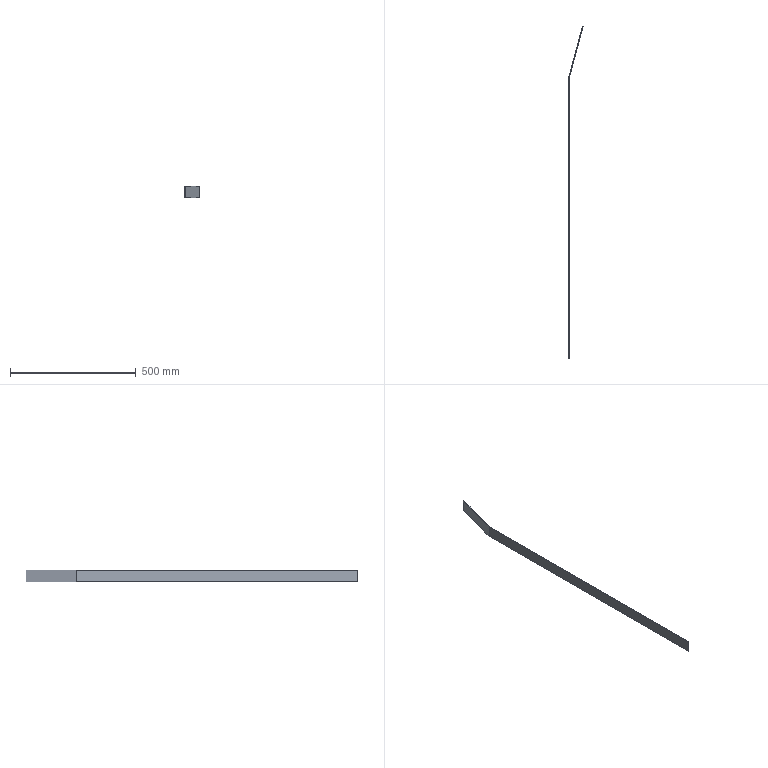Part | STEP file | SN10_016_001-01_CHAPA | 1 solid | 10 faces | box 56.488 x 1320 x 45 mm | volume 179098 mm3 | plane 8 | cylinder 2 | commonest cylinder face diameters 6 x1 12 x1
STEP:
#1=CARTESIAN_POINT('',(0.,0.,0.));
#2=DIRECTION('',(0.,0.,1.));
#3=DIRECTION('',(1.,0.,0.));
#4=AXIS2_PLACEMENT_3D('',#1,#2,#3);
#5=CARTESIAN_POINT('',(5319.204,-379.237,95.));
#6=VERTEX_POINT('',#5);
#7=CARTESIAN_POINT('',(5372.59,-180.,95.));
#8=VERTEX_POINT('',#7);
#9=CARTESIAN_POINT('',(5319.204,-379.237,95.));
#10=DIRECTION('',(0.2588,0.9659,0.));
#11=VECTOR('',#10,1.);
#12=LINE('',#9,#11);
#13=CARTESIAN_POINT('',(5319.204,-379.237,45.));
#14=DIRECTION('',(0.9659,-0.2588,0.));
#15=DIRECTION('',(0.,0.,-1.));
#16=AXIS2_PLACEMENT_3D('',#13,#14,#15);
#17=PLANE('',#16);
#18=CARTESIAN_POINT('',(-50.,0.));
#19=DIRECTION('',(0.,1.));
#20=VECTOR('',#19,1.);
#21=LINE('',#18,#20);
#22=(GEOMETRIC_REPRESENTATION_CONTEXT(2)PARAMETRIC_REPRESENTATION_CONTEXT()REPRESENTATION_CONTEXT('',''));
#23=DEFINITIONAL_REPRESENTATION('',(#21),#22);
#24=PCURVE('',#17,#23);
#25=CARTESIAN_POINT('',(0.,0.,95.));
#26=DIRECTION('',(0.,0.,1.));
#27=DIRECTION('',(1.,0.,0.));
#28=AXIS2_PLACEMENT_3D('',#25,#26,#27);
#29=PLANE('',#28);
#30=CARTESIAN_POINT('',(5319.204,-379.237));
#31=DIRECTION('',(0.2588,0.9659));
#32=VECTOR('',#31,1.);
#33=LINE('',#30,#32);
#34=(GEOMETRIC_REPRESENTATION_CONTEXT(2)PARAMETRIC_REPRESENTATION_CONTEXT()REPRESENTATION_CONTEXT('',''));
#35=DEFINITIONAL_REPRESENTATION('',(#33),#34);
#36=PCURVE('',#29,#35);
#37=SURFACE_CURVE('',#12,(#24,#36),.PCURVE_S1.);
#38=EDGE_CURVE('',#6,#8,#37,.T.);
#39=ORIENTED_EDGE('',*,*,#38,.T.);
#40=CARTESIAN_POINT('',(5372.59,-180.,50.));
#41=VERTEX_POINT('',#40);
#42=CARTESIAN_POINT('',(5372.59,-180.,50.));
#43=DIRECTION('',(0.,0.,1.));
#44=VECTOR('',#43,1.);
#45=LINE('',#42,#44);
#46=CARTESIAN_POINT('',(-5.,206.265));
#47=DIRECTION('',(-1.,0.));
#48=VECTOR('',#47,1.);
#49=LINE('',#46,#48);
#50=(GEOMETRIC_REPRESENTATION_CONTEXT(2)PARAMETRIC_REPRESENTATION_CONTEXT()REPRESENTATION_CONTEXT('',''));
#51=DEFINITIONAL_REPRESENTATION('',(#49),#50);
#52=PCURVE('',#17,#51);
#53=CARTESIAN_POINT('',(5375.488,-180.776,45.));
#54=DIRECTION('',(0.2588,0.9659,0.));
#55=DIRECTION('',(0.,0.,1.));
#56=AXIS2_PLACEMENT_3D('',#53,#54,#55);
#57=PLANE('',#56);
#58=CARTESIAN_POINT('',(5.,-3.));
#59=DIRECTION('',(1.,0.));
#60=VECTOR('',#59,1.);
#61=LINE('',#58,#60);
#62=(GEOMETRIC_REPRESENTATION_CONTEXT(2)PARAMETRIC_REPRESENTATION_CONTEXT()REPRESENTATION_CONTEXT('',''));
#63=DEFINITIONAL_REPRESENTATION('',(#61),#62);
#64=PCURVE('',#57,#63);
#65=SURFACE_CURVE('',#45,(#52,#64),.PCURVE_S1.);
#66=EDGE_CURVE('',#41,#8,#65,.T.);
#67=ORIENTED_EDGE('',*,*,#66,.F.);
#68=CARTESIAN_POINT('',(5319.204,-379.237,50.));
#69=VERTEX_POINT('',#68);
#70=CARTESIAN_POINT('',(5319.204,-379.237,50.));
#71=DIRECTION('',(0.2588,0.9659,0.));
#72=VECTOR('',#71,1.);
#73=LINE('',#70,#72);
#74=CARTESIAN_POINT('',(-5.,0.));
#75=DIRECTION('',(0.,1.));
#76=VECTOR('',#75,1.);
#77=LINE('',#74,#76);
#78=(GEOMETRIC_REPRESENTATION_CONTEXT(2)PARAMETRIC_REPRESENTATION_CONTEXT()REPRESENTATION_CONTEXT('',''));
#79=DEFINITIONAL_REPRESENTATION('',(#77),#78);
#80=PCURVE('',#17,#79);
#81=CARTESIAN_POINT('',(0.,0.,50.));
#82=DIRECTION('',(0.,0.,1.));
#83=DIRECTION('',(1.,0.,0.));
#84=AXIS2_PLACEMENT_3D('',#81,#82,#83);
#85=PLANE('',#84);
#86=CARTESIAN_POINT('',(5319.204,-379.237));
#87=DIRECTION('',(0.2588,0.9659));
#88=VECTOR('',#87,1.);
#89=LINE('',#86,#88);
#90=(GEOMETRIC_REPRESENTATION_CONTEXT(2)PARAMETRIC_REPRESENTATION_CONTEXT()REPRESENTATION_CONTEXT('',''));
#91=DEFINITIONAL_REPRESENTATION('',(#89),#90);
#92=PCURVE('',#85,#91);
#93=SURFACE_CURVE('',#73,(#80,#92),.PCURVE_S1.);
#94=EDGE_CURVE('',#69,#41,#93,.T.);
#95=ORIENTED_EDGE('',*,*,#94,.F.);
#96=CARTESIAN_POINT('',(5319.204,-379.237,50.));
#97=DIRECTION('',(0.,0.,1.));
#98=VECTOR('',#97,1.);
#99=LINE('',#96,#98);
#100=CARTESIAN_POINT('',(-5.,0.));
#101=DIRECTION('',(-1.,0.));
#102=VECTOR('',#101,1.);
#103=LINE('',#100,#102);
#104=(GEOMETRIC_REPRESENTATION_CONTEXT(2)PARAMETRIC_REPRESENTATION_CONTEXT()REPRESENTATION_CONTEXT('',''));
#105=DEFINITIONAL_REPRESENTATION('',(#103),#104);
#106=PCURVE('',#17,#105);
#107=CARTESIAN_POINT('',(5325.,-380.79,72.5));
#108=DIRECTION('',(0.,0.,1.));
#109=DIRECTION('',(-0.9659,0.2588,0.));
#110=AXIS2_PLACEMENT_3D('',#107,#108,#109);
#111=CYLINDRICAL_SURFACE('',#110,6.);
#112=CARTESIAN_POINT('',(0.,-22.5));
#113=DIRECTION('',(0.,1.));
#114=VECTOR('',#113,1.);
#115=LINE('',#112,#114);
#116=(GEOMETRIC_REPRESENTATION_CONTEXT(2)PARAMETRIC_REPRESENTATION_CONTEXT()REPRESENTATION_CONTEXT('',''));
#117=DEFINITIONAL_REPRESENTATION('',(#115),#116);
#118=PCURVE('',#111,#117);
#119=SURFACE_CURVE('',#99,(#106,#118),.PCURVE_S1.);
#120=EDGE_CURVE('',#69,#6,#119,.T.);
#121=ORIENTED_EDGE('',*,*,#120,.T.);
#122=EDGE_LOOP('',(#39,#67,#95,#121));
#123=FACE_BOUND('',#122,.T.);
#124=ADVANCED_FACE('',(#123),#17,.F.);
#125=ORIENTED_EDGE('',*,*,#120,.F.);
#126=CARTESIAN_POINT('',(5319.,-380.79,50.));
#127=VERTEX_POINT('',#126);
#128=CARTESIAN_POINT('',(5325.,-380.79,50.));
#129=DIRECTION('',(0.,0.,1.));
#130=DIRECTION('',(1.,0.,0.));
#131=AXIS2_PLACEMENT_3D('',#128,#129,#130);
#132=CIRCLE('',#131,6.);
#133=CARTESIAN_POINT('',(-2.88,-22.5));
#134=DIRECTION('',(1.,0.));
#135=VECTOR('',#134,1.);
#136=LINE('',#133,#135);
#137=(GEOMETRIC_REPRESENTATION_CONTEXT(2)PARAMETRIC_REPRESENTATION_CONTEXT()REPRESENTATION_CONTEXT('',''));
#138=DEFINITIONAL_REPRESENTATION('',(#136),#137);
#139=PCURVE('',#111,#138);
#140=CARTESIAN_POINT('',(5325.,-380.79));
#141=DIRECTION('',(1.,0.));
#142=AXIS2_PLACEMENT_2D('',#140,#141);
#143=CIRCLE('',#142,6.);
#144=(GEOMETRIC_REPRESENTATION_CONTEXT(2)PARAMETRIC_REPRESENTATION_CONTEXT()REPRESENTATION_CONTEXT('',''));
#145=DEFINITIONAL_REPRESENTATION('',(#143),#144);
#146=PCURVE('',#85,#145);
#147=SURFACE_CURVE('',#132,(#139,#146),.PCURVE_S1.);
#148=EDGE_CURVE('',#69,#127,#147,.T.);
#149=ORIENTED_EDGE('',*,*,#148,.T.);
#150=CARTESIAN_POINT('',(5319.,-380.79,95.));
#151=VERTEX_POINT('',#150);
#152=CARTESIAN_POINT('',(5319.,-380.79,50.));
#153=DIRECTION('',(0.,0.,1.));
#154=VECTOR('',#153,1.);
#155=LINE('',#152,#154);
#156=CARTESIAN_POINT('',(0.2618,-22.5));
#157=DIRECTION('',(0.,1.));
#158=VECTOR('',#157,1.);
#159=LINE('',#156,#158);
#160=(GEOMETRIC_REPRESENTATION_CONTEXT(2)PARAMETRIC_REPRESENTATION_CONTEXT()REPRESENTATION_CONTEXT('',''));
#161=DEFINITIONAL_REPRESENTATION('',(#159),#160);
#162=PCURVE('',#111,#161);
#163=CARTESIAN_POINT('',(5319.,-1500.,45.));
#164=DIRECTION('',(1.,0.,0.));
#165=DIRECTION('',(0.,0.,-1.));
#166=AXIS2_PLACEMENT_3D('',#163,#164,#165);
#167=PLANE('',#166);
#168=CARTESIAN_POINT('',(-5.,1119.21));
#169=DIRECTION('',(-1.,0.));
#170=VECTOR('',#169,1.);
#171=LINE('',#168,#170);
#172=(GEOMETRIC_REPRESENTATION_CONTEXT(2)PARAMETRIC_REPRESENTATION_CONTEXT()REPRESENTATION_CONTEXT('',''));
#173=DEFINITIONAL_REPRESENTATION('',(#171),#172);
#174=PCURVE('',#167,#173);
#175=SURFACE_CURVE('',#155,(#162,#174),.PCURVE_S1.);
#176=EDGE_CURVE('',#127,#151,#175,.T.);
#177=ORIENTED_EDGE('',*,*,#176,.T.);
#178=CARTESIAN_POINT('',(5325.,-380.79,95.));
#179=DIRECTION('',(0.,0.,1.));
#180=DIRECTION('',(1.,0.,0.));
#181=AXIS2_PLACEMENT_3D('',#178,#179,#180);
#182=CIRCLE('',#181,6.);
#183=CARTESIAN_POINT('',(-2.88,22.5));
#184=DIRECTION('',(1.,0.));
#185=VECTOR('',#184,1.);
#186=LINE('',#183,#185);
#187=(GEOMETRIC_REPRESENTATION_CONTEXT(2)PARAMETRIC_REPRESENTATION_CONTEXT()REPRESENTATION_CONTEXT('',''));
#188=DEFINITIONAL_REPRESENTATION('',(#186),#187);
#189=PCURVE('',#111,#188);
#190=CARTESIAN_POINT('',(5325.,-380.79));
#191=DIRECTION('',(1.,0.));
#192=AXIS2_PLACEMENT_2D('',#190,#191);
#193=CIRCLE('',#192,6.);
#194=(GEOMETRIC_REPRESENTATION_CONTEXT(2)PARAMETRIC_REPRESENTATION_CONTEXT()REPRESENTATION_CONTEXT('',''));
#195=DEFINITIONAL_REPRESENTATION('',(#193),#194);
#196=PCURVE('',#29,#195);
#197=SURFACE_CURVE('',#182,(#189,#196),.PCURVE_S1.);
#198=EDGE_CURVE('',#6,#151,#197,.T.);
#199=ORIENTED_EDGE('',*,*,#198,.F.);
#200=EDGE_LOOP('',(#125,#149,#177,#199));
#201=FACE_BOUND('',#200,.T.);
#202=ADVANCED_FACE('',(#201),#111,.T.);
#203=CARTESIAN_POINT('',(5319.,-1500.,95.));
#204=VERTEX_POINT('',#203);
#205=CARTESIAN_POINT('',(5319.,-1500.,95.));
#206=DIRECTION('',(0.,1.,0.));
#207=VECTOR('',#206,1.);
#208=LINE('',#205,#207);
#209=CARTESIAN_POINT('',(-50.,0.));
#210=DIRECTION('',(0.,1.));
#211=VECTOR('',#210,1.);
#212=LINE('',#209,#211);
#213=(GEOMETRIC_REPRESENTATION_CONTEXT(2)PARAMETRIC_REPRESENTATION_CONTEXT()REPRESENTATION_CONTEXT('',''));
#214=DEFINITIONAL_REPRESENTATION('',(#212),#213);
#215=PCURVE('',#167,#214);
#216=CARTESIAN_POINT('',(5319.,-1500.));
#217=DIRECTION('',(0.,1.));
#218=VECTOR('',#217,1.);
#219=LINE('',#216,#218);
#220=(GEOMETRIC_REPRESENTATION_CONTEXT(2)PARAMETRIC_REPRESENTATION_CONTEXT()REPRESENTATION_CONTEXT('',''));
#221=DEFINITIONAL_REPRESENTATION('',(#219),#220);
#222=PCURVE('',#29,#221);
#223=SURFACE_CURVE('',#208,(#215,#222),.PCURVE_S1.);
#224=EDGE_CURVE('',#204,#151,#223,.T.);
#225=ORIENTED_EDGE('',*,*,#224,.T.);
#226=ORIENTED_EDGE('',*,*,#176,.F.);
#227=CARTESIAN_POINT('',(5319.,-1500.,50.));
#228=VERTEX_POINT('',#227);
#229=CARTESIAN_POINT('',(5319.,-1500.,50.));
#230=DIRECTION('',(0.,1.,0.));
#231=VECTOR('',#230,1.);
#232=LINE('',#229,#231);
#233=CARTESIAN_POINT('',(-5.,0.));
#234=DIRECTION('',(0.,1.));
#235=VECTOR('',#234,1.);
#236=LINE('',#233,#235);
#237=(GEOMETRIC_REPRESENTATION_CONTEXT(2)PARAMETRIC_REPRESENTATION_CONTEXT()REPRESENTATION_CONTEXT('',''));
#238=DEFINITIONAL_REPRESENTATION('',(#236),#237);
#239=PCURVE('',#167,#238);
#240=CARTESIAN_POINT('',(5319.,-1500.));
#241=DIRECTION('',(0.,1.));
#242=VECTOR('',#241,1.);
#243=LINE('',#240,#242);
#244=(GEOMETRIC_REPRESENTATION_CONTEXT(2)PARAMETRIC_REPRESENTATION_CONTEXT()REPRESENTATION_CONTEXT('',''));
#245=DEFINITIONAL_REPRESENTATION('',(#243),#244);
#246=PCURVE('',#85,#245);
#247=SURFACE_CURVE('',#232,(#239,#246),.PCURVE_S1.);
#248=EDGE_CURVE('',#228,#127,#247,.T.);
#249=ORIENTED_EDGE('',*,*,#248,.F.);
#250=CARTESIAN_POINT('',(5319.,-1500.,50.));
#251=DIRECTION('',(0.,0.,1.));
#252=VECTOR('',#251,1.);
#253=LINE('',#250,#252);
#254=CARTESIAN_POINT('',(-5.,0.));
#255=DIRECTION('',(-1.,0.));
#256=VECTOR('',#255,1.);
#257=LINE('',#254,#256);
#258=(GEOMETRIC_REPRESENTATION_CONTEXT(2)PARAMETRIC_REPRESENTATION_CONTEXT()REPRESENTATION_CONTEXT('',''));
#259=DEFINITIONAL_REPRESENTATION('',(#257),#258);
#260=PCURVE('',#167,#259);
#261=CARTESIAN_POINT('',(5319.,-1500.,45.));
#262=DIRECTION('',(0.,-1.,0.));
#263=DIRECTION('',(0.,0.,-1.));
#264=AXIS2_PLACEMENT_3D('',#261,#262,#263);
#265=PLANE('',#264);
#266=CARTESIAN_POINT('',(-5.,0.));
#267=DIRECTION('',(-1.,0.));
#268=VECTOR('',#267,1.);
#269=LINE('',#266,#268);
#270=(GEOMETRIC_REPRESENTATION_CONTEXT(2)PARAMETRIC_REPRESENTATION_CONTEXT()REPRESENTATION_CONTEXT('',''));
#271=DEFINITIONAL_REPRESENTATION('',(#269),#270);
#272=PCURVE('',#265,#271);
#273=SURFACE_CURVE('',#253,(#260,#272),.PCURVE_S1.);
#274=EDGE_CURVE('',#228,#204,#273,.T.);
#275=ORIENTED_EDGE('',*,*,#274,.T.);
#276=EDGE_LOOP('',(#225,#226,#249,#275));
#277=FACE_BOUND('',#276,.T.);
#278=ADVANCED_FACE('',(#277),#167,.F.);
#279=ORIENTED_EDGE('',*,*,#274,.F.);
#280=CARTESIAN_POINT('',(5322.,-1500.,50.));
#281=VERTEX_POINT('',#280);
#282=CARTESIAN_POINT('',(5319.,-1500.,50.));
#283=DIRECTION('',(1.,0.,0.));
#284=VECTOR('',#283,1.);
#285=LINE('',#282,#284);
#286=CARTESIAN_POINT('',(-5.,0.));
#287=DIRECTION('',(0.,1.));
#288=VECTOR('',#287,1.);
#289=LINE('',#286,#288);
#290=(GEOMETRIC_REPRESENTATION_CONTEXT(2)PARAMETRIC_REPRESENTATION_CONTEXT()REPRESENTATION_CONTEXT('',''));
#291=DEFINITIONAL_REPRESENTATION('',(#289),#290);
#292=PCURVE('',#265,#291);
#293=CARTESIAN_POINT('',(5319.,-1500.));
#294=DIRECTION('',(1.,0.));
#295=VECTOR('',#294,1.);
#296=LINE('',#293,#295);
#297=(GEOMETRIC_REPRESENTATION_CONTEXT(2)PARAMETRIC_REPRESENTATION_CONTEXT()REPRESENTATION_CONTEXT('',''));
#298=DEFINITIONAL_REPRESENTATION('',(#296),#297);
#299=PCURVE('',#85,#298);
#300=SURFACE_CURVE('',#285,(#292,#299),.PCURVE_S1.);
#301=EDGE_CURVE('',#228,#281,#300,.T.);
#302=ORIENTED_EDGE('',*,*,#301,.T.);
#303=CARTESIAN_POINT('',(5322.,-1500.,95.));
#304=VERTEX_POINT('',#303);
#305=CARTESIAN_POINT('',(5322.,-1500.,50.));
#306=DIRECTION('',(0.,0.,1.));
#307=VECTOR('',#306,1.);
#308=LINE('',#305,#307);
#309=CARTESIAN_POINT('',(-5.,3.));
#310=DIRECTION('',(-1.,0.));
#311=VECTOR('',#310,1.);
#312=LINE('',#309,#311);
#313=(GEOMETRIC_REPRESENTATION_CONTEXT(2)PARAMETRIC_REPRESENTATION_CONTEXT()REPRESENTATION_CONTEXT('',''));
#314=DEFINITIONAL_REPRESENTATION('',(#312),#313);
#315=PCURVE('',#265,#314);
#316=CARTESIAN_POINT('',(5322.,-1500.,45.));
#317=DIRECTION('',(1.,0.,0.));
#318=DIRECTION('',(0.,0.,-1.));
#319=AXIS2_PLACEMENT_3D('',#316,#317,#318);
#320=PLANE('',#319);
#321=CARTESIAN_POINT('',(-5.,0.));
#322=DIRECTION('',(-1.,0.));
#323=VECTOR('',#322,1.);
#324=LINE('',#321,#323);
#325=(GEOMETRIC_REPRESENTATION_CONTEXT(2)PARAMETRIC_REPRESENTATION_CONTEXT()REPRESENTATION_CONTEXT('',''));
#326=DEFINITIONAL_REPRESENTATION('',(#324),#325);
#327=PCURVE('',#320,#326);
#328=SURFACE_CURVE('',#308,(#315,#327),.PCURVE_S1.);
#329=EDGE_CURVE('',#281,#304,#328,.T.);
#330=ORIENTED_EDGE('',*,*,#329,.T.);
#331=CARTESIAN_POINT('',(5319.,-1500.,95.));
#332=DIRECTION('',(1.,0.,0.));
#333=VECTOR('',#332,1.);
#334=LINE('',#331,#333);
#335=CARTESIAN_POINT('',(-50.,0.));
#336=DIRECTION('',(0.,1.));
#337=VECTOR('',#336,1.);
#338=LINE('',#335,#337);
#339=(GEOMETRIC_REPRESENTATION_CONTEXT(2)PARAMETRIC_REPRESENTATION_CONTEXT()REPRESENTATION_CONTEXT('',''));
#340=DEFINITIONAL_REPRESENTATION('',(#338),#339);
#341=PCURVE('',#265,#340);
#342=CARTESIAN_POINT('',(5319.,-1500.));
#343=DIRECTION('',(1.,0.));
#344=VECTOR('',#343,1.);
#345=LINE('',#342,#344);
#346=(GEOMETRIC_REPRESENTATION_CONTEXT(2)PARAMETRIC_REPRESENTATION_CONTEXT()REPRESENTATION_CONTEXT('',''));
#347=DEFINITIONAL_REPRESENTATION('',(#345),#346);
#348=PCURVE('',#29,#347);
#349=SURFACE_CURVE('',#334,(#341,#348),.PCURVE_S1.);
#350=EDGE_CURVE('',#204,#304,#349,.T.);
#351=ORIENTED_EDGE('',*,*,#350,.F.);
#352=EDGE_LOOP('',(#279,#302,#330,#351));
#353=FACE_BOUND('',#352,.T.);
#354=ADVANCED_FACE('',(#353),#265,.T.);
#355=ORIENTED_EDGE('',*,*,#329,.F.);
#356=CARTESIAN_POINT('',(5322.,-380.79,50.));
#357=VERTEX_POINT('',#356);
#358=CARTESIAN_POINT('',(5322.,-1500.,50.));
#359=DIRECTION('',(0.,1.,0.));
#360=VECTOR('',#359,1.);
#361=LINE('',#358,#360);
#362=CARTESIAN_POINT('',(-5.,0.));
#363=DIRECTION('',(0.,1.));
#364=VECTOR('',#363,1.);
#365=LINE('',#362,#364);
#366=(GEOMETRIC_REPRESENTATION_CONTEXT(2)PARAMETRIC_REPRESENTATION_CONTEXT()REPRESENTATION_CONTEXT('',''));
#367=DEFINITIONAL_REPRESENTATION('',(#365),#366);
#368=PCURVE('',#320,#367);
#369=CARTESIAN_POINT('',(5322.,-1500.));
#370=DIRECTION('',(0.,1.));
#371=VECTOR('',#370,1.);
#372=LINE('',#369,#371);
#373=(GEOMETRIC_REPRESENTATION_CONTEXT(2)PARAMETRIC_REPRESENTATION_CONTEXT()REPRESENTATION_CONTEXT('',''));
#374=DEFINITIONAL_REPRESENTATION('',(#372),#373);
#375=PCURVE('',#85,#374);
#376=SURFACE_CURVE('',#361,(#368,#375),.PCURVE_S1.);
#377=EDGE_CURVE('',#281,#357,#376,.T.);
#378=ORIENTED_EDGE('',*,*,#377,.T.);
#379=CARTESIAN_POINT('',(5322.,-380.79,95.));
#380=VERTEX_POINT('',#379);
#381=CARTESIAN_POINT('',(5322.,-380.79,50.));
#382=DIRECTION('',(0.,0.,1.));
#383=VECTOR('',#382,1.);
#384=LINE('',#381,#383);
#385=CARTESIAN_POINT('',(-5.,1119.21));
#386=DIRECTION('',(-1.,0.));
#387=VECTOR('',#386,1.);
#388=LINE('',#385,#387);
#389=(GEOMETRIC_REPRESENTATION_CONTEXT(2)PARAMETRIC_REPRESENTATION_CONTEXT()REPRESENTATION_CONTEXT('',''));
#390=DEFINITIONAL_REPRESENTATION('',(#388),#389);
#391=PCURVE('',#320,#390);
#392=CARTESIAN_POINT('',(5325.,-380.79,72.5));
#393=DIRECTION('',(0.,0.,1.));
#394=DIRECTION('',(-0.9659,0.2588,0.));
#395=AXIS2_PLACEMENT_3D('',#392,#393,#394);
#396=CYLINDRICAL_SURFACE('',#395,3.);
#397=CARTESIAN_POINT('',(0.2618,-22.5));
#398=DIRECTION('',(0.,1.));
#399=VECTOR('',#398,1.);
#400=LINE('',#397,#399);
#401=(GEOMETRIC_REPRESENTATION_CONTEXT(2)PARAMETRIC_REPRESENTATION_CONTEXT()REPRESENTATION_CONTEXT('',''));
#402=DEFINITIONAL_REPRESENTATION('',(#400),#401);
#403=PCURVE('',#396,#402);
#404=SURFACE_CURVE('',#384,(#391,#403),.PCURVE_S1.);
#405=EDGE_CURVE('',#357,#380,#404,.T.);
#406=ORIENTED_EDGE('',*,*,#405,.T.);
#407=CARTESIAN_POINT('',(5322.,-1500.,95.));
#408=DIRECTION('',(0.,1.,0.));
#409=VECTOR('',#408,1.);
#410=LINE('',#407,#409);
#411=CARTESIAN_POINT('',(-50.,0.));
#412=DIRECTION('',(0.,1.));
#413=VECTOR('',#412,1.);
#414=LINE('',#411,#413);
#415=(GEOMETRIC_REPRESENTATION_CONTEXT(2)PARAMETRIC_REPRESENTATION_CONTEXT()REPRESENTATION_CONTEXT('',''));
#416=DEFINITIONAL_REPRESENTATION('',(#414),#415);
#417=PCURVE('',#320,#416);
#418=CARTESIAN_POINT('',(5322.,-1500.));
#419=DIRECTION('',(0.,1.));
#420=VECTOR('',#419,1.);
#421=LINE('',#418,#420);
#422=(GEOMETRIC_REPRESENTATION_CONTEXT(2)PARAMETRIC_REPRESENTATION_CONTEXT()REPRESENTATION_CONTEXT('',''));
#423=DEFINITIONAL_REPRESENTATION('',(#421),#422);
#424=PCURVE('',#29,#423);
#425=SURFACE_CURVE('',#410,(#417,#424),.PCURVE_S1.);
#426=EDGE_CURVE('',#304,#380,#425,.T.);
#427=ORIENTED_EDGE('',*,*,#426,.F.);
#428=EDGE_LOOP('',(#355,#378,#406,#427));
#429=FACE_BOUND('',#428,.T.);
#430=ADVANCED_FACE('',(#429),#320,.T.);
#431=CARTESIAN_POINT('',(5322.102,-380.013,50.));
#432=VERTEX_POINT('',#431);
#433=CARTESIAN_POINT('',(5322.102,-380.013,95.));
#434=VERTEX_POINT('',#433);
#435=CARTESIAN_POINT('',(5322.102,-380.013,50.));
#436=DIRECTION('',(0.,0.,1.));
#437=VECTOR('',#436,1.);
#438=LINE('',#435,#437);
#439=CARTESIAN_POINT('',(0.,-22.5));
#440=DIRECTION('',(0.,1.));
#441=VECTOR('',#440,1.);
#442=LINE('',#439,#441);
#443=(GEOMETRIC_REPRESENTATION_CONTEXT(2)PARAMETRIC_REPRESENTATION_CONTEXT()REPRESENTATION_CONTEXT('',''));
#444=DEFINITIONAL_REPRESENTATION('',(#442),#443);
#445=PCURVE('',#396,#444);
#446=CARTESIAN_POINT('',(5322.102,-380.013,45.));
#447=DIRECTION('',(0.9659,-0.2588,0.));
#448=DIRECTION('',(0.,0.,-1.));
#449=AXIS2_PLACEMENT_3D('',#446,#447,#448);
#450=PLANE('',#449);
#451=CARTESIAN_POINT('',(-5.,0.));
#452=DIRECTION('',(-1.,0.));
#453=VECTOR('',#452,1.);
#454=LINE('',#451,#453);
#455=(GEOMETRIC_REPRESENTATION_CONTEXT(2)PARAMETRIC_REPRESENTATION_CONTEXT()REPRESENTATION_CONTEXT('',''));
#456=DEFINITIONAL_REPRESENTATION('',(#454),#455);
#457=PCURVE('',#450,#456);
#458=SURFACE_CURVE('',#438,(#445,#457),.PCURVE_S1.);
#459=EDGE_CURVE('',#432,#434,#458,.T.);
#460=ORIENTED_EDGE('',*,*,#459,.F.);
#461=CARTESIAN_POINT('',(5325.,-380.79,50.));
#462=DIRECTION('',(0.,0.,1.));
#463=DIRECTION('',(1.,0.,0.));
#464=AXIS2_PLACEMENT_3D('',#461,#462,#463);
#465=CIRCLE('',#464,3.);
#466=CARTESIAN_POINT('',(-2.88,-22.5));
#467=DIRECTION('',(1.,0.));
#468=VECTOR('',#467,1.);
#469=LINE('',#466,#468);
#470=(GEOMETRIC_REPRESENTATION_CONTEXT(2)PARAMETRIC_REPRESENTATION_CONTEXT()REPRESENTATION_CONTEXT('',''));
#471=DEFINITIONAL_REPRESENTATION('',(#469),#470);
#472=PCURVE('',#396,#471);
#473=CARTESIAN_POINT('',(5325.,-380.79));
#474=DIRECTION('',(1.,0.));
#475=AXIS2_PLACEMENT_2D('',#473,#474);
#476=CIRCLE('',#475,3.);
#477=(GEOMETRIC_REPRESENTATION_CONTEXT(2)PARAMETRIC_REPRESENTATION_CONTEXT()REPRESENTATION_CONTEXT('',''));
#478=DEFINITIONAL_REPRESENTATION('',(#476),#477);
#479=PCURVE('',#85,#478);
#480=SURFACE_CURVE('',#465,(#472,#479),.PCURVE_S1.);
#481=EDGE_CURVE('',#432,#357,#480,.T.);
#482=ORIENTED_EDGE('',*,*,#481,.T.);
#483=ORIENTED_EDGE('',*,*,#405,.T.);
#484=CARTESIAN_POINT('',(5325.,-380.79,95.));
#485=DIRECTION('',(0.,0.,1.));
#486=DIRECTION('',(1.,0.,0.));
#487=AXIS2_PLACEMENT_3D('',#484,#485,#486);
#488=CIRCLE('',#487,3.);
#489=CARTESIAN_POINT('',(-2.88,22.5));
#490=DIRECTION('',(1.,0.));
#491=VECTOR('',#490,1.);
#492=LINE('',#489,#491);
#493=(GEOMETRIC_REPRESENTATION_CONTEXT(2)PARAMETRIC_REPRESENTATION_CONTEXT()REPRESENTATION_CONTEXT('',''));
#494=DEFINITIONAL_REPRESENTATION('',(#492),#493);
#495=PCURVE('',#396,#494);
#496=CARTESIAN_POINT('',(5325.,-380.79));
#497=DIRECTION('',(1.,0.));
#498=AXIS2_PLACEMENT_2D('',#496,#497);
#499=CIRCLE('',#498,3.);
#500=(GEOMETRIC_REPRESENTATION_CONTEXT(2)PARAMETRIC_REPRESENTATION_CONTEXT()REPRESENTATION_CONTEXT('',''));
#501=DEFINITIONAL_REPRESENTATION('',(#499),#500);
#502=PCURVE('',#29,#501);
#503=SURFACE_CURVE('',#488,(#495,#502),.PCURVE_S1.);
#504=EDGE_CURVE('',#434,#380,#503,.T.);
#505=ORIENTED_EDGE('',*,*,#504,.F.);
#506=EDGE_LOOP('',(#460,#482,#483,#505));
#507=FACE_BOUND('',#506,.F.);
#508=ADVANCED_FACE('',(#507),#396,.F.);
#509=ORIENTED_EDGE('',*,*,#459,.F.);
#510=CARTESIAN_POINT('',(5375.488,-180.776,50.));
#511=VERTEX_POINT('',#510);
#512=CARTESIAN_POINT('',(5322.102,-380.013,50.));
#513=DIRECTION('',(0.2588,0.9659,0.));
#514=VECTOR('',#513,1.);
#515=LINE('',#512,#514);
#516=CARTESIAN_POINT('',(-5.,0.));
#517=DIRECTION('',(0.,1.));
#518=VECTOR('',#517,1.);
#519=LINE('',#516,#518);
#520=(GEOMETRIC_REPRESENTATION_CONTEXT(2)PARAMETRIC_REPRESENTATION_CONTEXT()REPRESENTATION_CONTEXT('',''));
#521=DEFINITIONAL_REPRESENTATION('',(#519),#520);
#522=PCURVE('',#450,#521);
#523=CARTESIAN_POINT('',(5322.102,-380.013));
#524=DIRECTION('',(0.2588,0.9659));
#525=VECTOR('',#524,1.);
#526=LINE('',#523,#525);
#527=(GEOMETRIC_REPRESENTATION_CONTEXT(2)PARAMETRIC_REPRESENTATION_CONTEXT()REPRESENTATION_CONTEXT('',''));
#528=DEFINITIONAL_REPRESENTATION('',(#526),#527);
#529=PCURVE('',#85,#528);
#530=SURFACE_CURVE('',#515,(#522,#529),.PCURVE_S1.);
#531=EDGE_CURVE('',#432,#511,#530,.T.);
#532=ORIENTED_EDGE('',*,*,#531,.T.);
#533=CARTESIAN_POINT('',(5375.488,-180.776,95.));
#534=VERTEX_POINT('',#533);
#535=CARTESIAN_POINT('',(5375.488,-180.776,50.));
#536=DIRECTION('',(0.,0.,1.));
#537=VECTOR('',#536,1.);
#538=LINE('',#535,#537);
#539=CARTESIAN_POINT('',(-5.,206.265));
#540=DIRECTION('',(-1.,0.));
#541=VECTOR('',#540,1.);
#542=LINE('',#539,#541);
#543=(GEOMETRIC_REPRESENTATION_CONTEXT(2)PARAMETRIC_REPRESENTATION_CONTEXT()REPRESENTATION_CONTEXT('',''));
#544=DEFINITIONAL_REPRESENTATION('',(#542),#543);
#545=PCURVE('',#450,#544);
#546=CARTESIAN_POINT('',(5.,0.));
#547=DIRECTION('',(1.,0.));
#548=VECTOR('',#547,1.);
#549=LINE('',#546,#548);
#550=(GEOMETRIC_REPRESENTATION_CONTEXT(2)PARAMETRIC_REPRESENTATION_CONTEXT()REPRESENTATION_CONTEXT('',''));
#551=DEFINITIONAL_REPRESENTATION('',(#549),#550);
#552=PCURVE('',#57,#551);
#553=SURFACE_CURVE('',#538,(#545,#552),.PCURVE_S1.);
#554=EDGE_CURVE('',#511,#534,#553,.T.);
#555=ORIENTED_EDGE('',*,*,#554,.T.);
#556=CARTESIAN_POINT('',(5322.102,-380.013,95.));
#557=DIRECTION('',(0.2588,0.9659,0.));
#558=VECTOR('',#557,1.);
#559=LINE('',#556,#558);
#560=CARTESIAN_POINT('',(-50.,0.));
#561=DIRECTION('',(0.,1.));
#562=VECTOR('',#561,1.);
#563=LINE('',#560,#562);
#564=(GEOMETRIC_REPRESENTATION_CONTEXT(2)PARAMETRIC_REPRESENTATION_CONTEXT()REPRESENTATION_CONTEXT('',''));
#565=DEFINITIONAL_REPRESENTATION('',(#563),#564);
#566=PCURVE('',#450,#565);
#567=CARTESIAN_POINT('',(5322.102,-380.013));
#568=DIRECTION('',(0.2588,0.9659));
#569=VECTOR('',#568,1.);
#570=LINE('',#567,#569);
#571=(GEOMETRIC_REPRESENTATION_CONTEXT(2)PARAMETRIC_REPRESENTATION_CONTEXT()REPRESENTATION_CONTEXT('',''));
#572=DEFINITIONAL_REPRESENTATION('',(#570),#571);
#573=PCURVE('',#29,#572);
#574=SURFACE_CURVE('',#559,(#566,#573),.PCURVE_S1.);
#575=EDGE_CURVE('',#434,#534,#574,.T.);
#576=ORIENTED_EDGE('',*,*,#575,.F.);
#577=EDGE_LOOP('',(#509,#532,#555,#576));
#578=FACE_BOUND('',#577,.T.);
#579=ADVANCED_FACE('',(#578),#450,.T.);
#580=ORIENTED_EDGE('',*,*,#554,.F.);
#581=CARTESIAN_POINT('',(5375.488,-180.776,50.));
#582=DIRECTION('',(-0.9659,0.2588,0.));
#583=VECTOR('',#582,1.);
#584=LINE('',#581,#583);
#585=CARTESIAN_POINT('',(5.,0.000000001));
#586=DIRECTION('',(0.,-1.));
#587=VECTOR('',#586,1.);
#588=LINE('',#585,#587);
#589=(GEOMETRIC_REPRESENTATION_CONTEXT(2)PARAMETRIC_REPRESENTATION_CONTEXT()REPRESENTATION_CONTEXT('',''));
#590=DEFINITIONAL_REPRESENTATION('',(#588),#589);
#591=PCURVE('',#57,#590);
#592=CARTESIAN_POINT('',(5375.488,-180.776));
#593=DIRECTION('',(-0.9659,0.2588));
#594=VECTOR('',#593,1.);
#595=LINE('',#592,#594);
#596=(GEOMETRIC_REPRESENTATION_CONTEXT(2)PARAMETRIC_REPRESENTATION_CONTEXT()REPRESENTATION_CONTEXT('',''));
#597=DEFINITIONAL_REPRESENTATION('',(#595),#596);
#598=PCURVE('',#85,#597);
#599=SURFACE_CURVE('',#584,(#591,#598),.PCURVE_S1.);
#600=EDGE_CURVE('',#511,#41,#599,.T.);
#601=ORIENTED_EDGE('',*,*,#600,.T.);
#602=ORIENTED_EDGE('',*,*,#66,.T.);
#603=CARTESIAN_POINT('',(5375.488,-180.776,95.));
#604=DIRECTION('',(-0.9659,0.2588,0.));
#605=VECTOR('',#604,1.);
#606=LINE('',#603,#605);
#607=CARTESIAN_POINT('',(50.,0.000000001));
#608=DIRECTION('',(0.,-1.));
#609=VECTOR('',#608,1.);
#610=LINE('',#607,#609);
#611=(GEOMETRIC_REPRESENTATION_CONTEXT(2)PARAMETRIC_REPRESENTATION_CONTEXT()REPRESENTATION_CONTEXT('',''));
#612=DEFINITIONAL_REPRESENTATION('',(#610),#611);
#613=PCURVE('',#57,#612);
#614=CARTESIAN_POINT('',(5375.488,-180.776));
#615=DIRECTION('',(-0.9659,0.2588));
#616=VECTOR('',#615,1.);
#617=LINE('',#614,#616);
#618=(GEOMETRIC_REPRESENTATION_CONTEXT(2)PARAMETRIC_REPRESENTATION_CONTEXT()REPRESENTATION_CONTEXT('',''));
#619=DEFINITIONAL_REPRESENTATION('',(#617),#618);
#620=PCURVE('',#29,#619);
#621=SURFACE_CURVE('',#606,(#613,#620),.PCURVE_S1.);
#622=EDGE_CURVE('',#534,#8,#621,.T.);
#623=ORIENTED_EDGE('',*,*,#622,.F.);
#624=EDGE_LOOP('',(#580,#601,#602,#623));
#625=FACE_BOUND('',#624,.T.);
#626=ADVANCED_FACE('',(#625),#57,.T.);
#627=ORIENTED_EDGE('',*,*,#600,.F.);
#628=ORIENTED_EDGE('',*,*,#531,.F.);
#629=ORIENTED_EDGE('',*,*,#481,.T.);
#630=ORIENTED_EDGE('',*,*,#377,.F.);
#631=ORIENTED_EDGE('',*,*,#301,.F.);
#632=ORIENTED_EDGE('',*,*,#248,.T.);
#633=ORIENTED_EDGE('',*,*,#148,.F.);
#634=ORIENTED_EDGE('',*,*,#94,.T.);
#635=EDGE_LOOP('',(#627,#628,#629,#630,#631,#632,#633,#634));
#636=FACE_BOUND('',#635,.T.);
#637=ADVANCED_FACE('',(#636),#85,.F.);
#638=ORIENTED_EDGE('',*,*,#38,.F.);
#639=ORIENTED_EDGE('',*,*,#198,.T.);
#640=ORIENTED_EDGE('',*,*,#224,.F.);
#641=ORIENTED_EDGE('',*,*,#350,.T.);
#642=ORIENTED_EDGE('',*,*,#426,.T.);
#643=ORIENTED_EDGE('',*,*,#504,.F.);
#644=ORIENTED_EDGE('',*,*,#575,.T.);
#645=ORIENTED_EDGE('',*,*,#622,.T.);
#646=EDGE_LOOP('',(#638,#639,#640,#641,#642,#643,#644,#645));
#647=FACE_BOUND('',#646,.T.);
#648=ADVANCED_FACE('',(#647),#29,.T.);
#649=CLOSED_SHELL('',(#124,#202,#278,#354,#430,#508,#579,#626,#637,#648));
#650=MANIFOLD_SOLID_BREP('',#649);
#651=(LENGTH_UNIT()NAMED_UNIT(*)SI_UNIT(.MILLI.,.METRE.));
#652=UNCERTAINTY_MEASURE_WITH_UNIT(LENGTH_MEASURE(0.0000001),#651,'','');
#653=(NAMED_UNIT(*)PLANE_ANGLE_UNIT()SI_UNIT($,.RADIAN.));
#654=(NAMED_UNIT(*)SI_UNIT($,.STERADIAN.)SOLID_ANGLE_UNIT());
#655=(GEOMETRIC_REPRESENTATION_CONTEXT(3)GLOBAL_UNCERTAINTY_ASSIGNED_CONTEXT((#652))GLOBAL_UNIT_ASSIGNED_CONTEXT((#651,#653,#654))REPRESENTATION_CONTEXT('',''));
#656=ADVANCED_BREP_SHAPE_REPRESENTATION('',(#4,#650),#655);